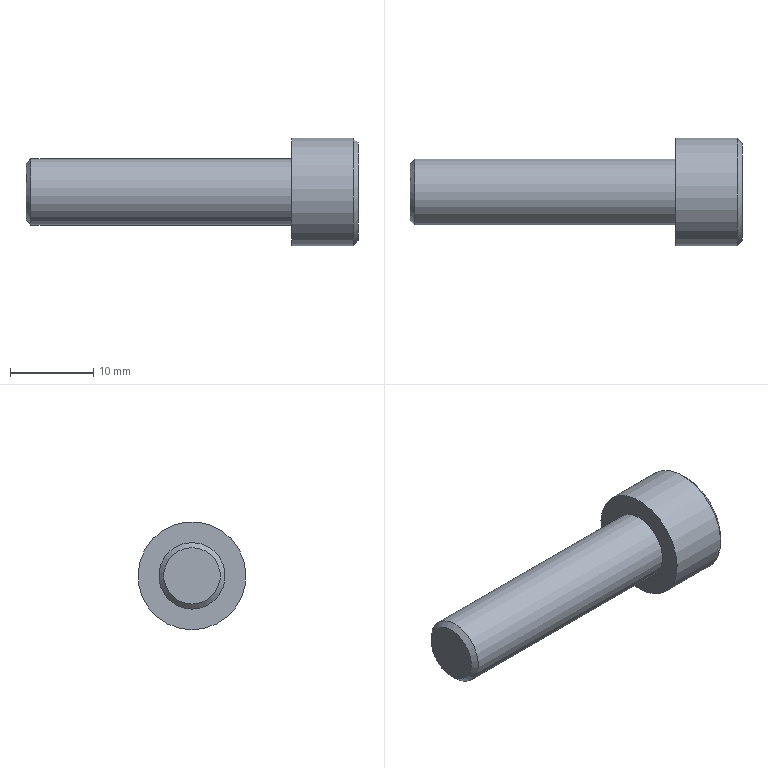Part | STEP file | solid 87 | 1 solid | 14 faces | box 40 x 13 x 13 mm | volume 2534 mm3 | plane 10 | cone 2 | cylinder 2 | commonest cylinder face diameters 8 x1 13 x1